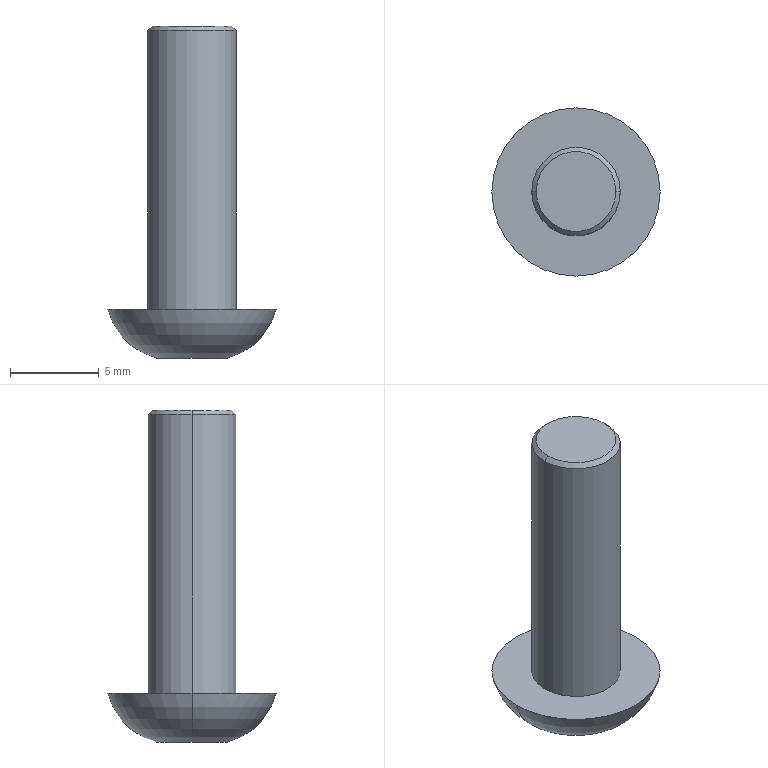Part | NX | features BREP 1 | 1 solid | 23 faces | box 9.5 x 9.5 x 18.75 mm | volume 434.554 mm3 | plane 15 | cone 4 | torus 2 | cylinder 2 | commonest cylinder face diameters 5 x2
STEP:
#1=CARTESIAN_POINT('',(0.,0.,-0.324));
#2=VERTEX_POINT('',#1);
#3=CARTESIAN_POINT('',(-1.5,0.,-1.19));
#4=VERTEX_POINT('',#3);
#5=CARTESIAN_POINT('',(-1.5,0.,-1.19));
#6=DIRECTION('',(-0.866,0.,-0.5));
#7=VECTOR('',#6,1000.);
#8=LINE('',#5,#7);
#9=EDGE_CURVE('',#2,#4,#8,.T.);
#10=ORIENTED_EDGE('',*,*,#9,.F.);
#11=CARTESIAN_POINT('',(1.5,0.,-1.19));
#12=VERTEX_POINT('',#11);
#13=CARTESIAN_POINT('',(1.5,0.,-1.19));
#14=DIRECTION('',(0.866,0.,-0.5));
#15=VECTOR('',#14,1000.);
#16=LINE('',#13,#15);
#17=EDGE_CURVE('',#2,#12,#16,.T.);
#18=ORIENTED_EDGE('',*,*,#17,.T.);
#19=CARTESIAN_POINT('',(1.299,-0.75,-1.19));
#20=VERTEX_POINT('',#19);
#21=CARTESIAN_POINT('',(0.,0.,-1.19));
#22=DIRECTION('',(0.,0.,1.));
#23=DIRECTION('',(1.,0.,0.));
#24=AXIS2_PLACEMENT_3D('',#21,#22,#23);
#25=CIRCLE('',#24,1.5);
#26=EDGE_CURVE('',#20,#12,#25,.T.);
#27=ORIENTED_EDGE('',*,*,#26,.F.);
#28=CARTESIAN_POINT('',(0.,-1.5,-1.19));
#29=VERTEX_POINT('',#28);
#30=CARTESIAN_POINT('',(0.,0.,-1.19));
#31=DIRECTION('',(0.,0.,1.));
#32=DIRECTION('',(1.,0.,0.));
#33=AXIS2_PLACEMENT_3D('',#30,#31,#32);
#34=CIRCLE('',#33,1.5);
#35=EDGE_CURVE('',#29,#20,#34,.T.);
#36=ORIENTED_EDGE('',*,*,#35,.F.);
#37=CARTESIAN_POINT('',(-1.299,-0.75,-1.19));
#38=VERTEX_POINT('',#37);
#39=CARTESIAN_POINT('',(0.,0.,-1.19));
#40=DIRECTION('',(0.,0.,1.));
#41=DIRECTION('',(1.,0.,0.));
#42=AXIS2_PLACEMENT_3D('',#39,#40,#41);
#43=CIRCLE('',#42,1.5);
#44=EDGE_CURVE('',#38,#29,#43,.T.);
#45=ORIENTED_EDGE('',*,*,#44,.F.);
#46=CARTESIAN_POINT('',(0.,0.,-1.19));
#47=DIRECTION('',(0.,0.,1.));
#48=DIRECTION('',(1.,0.,0.));
#49=AXIS2_PLACEMENT_3D('',#46,#47,#48);
#50=CIRCLE('',#49,1.5);
#51=EDGE_CURVE('',#4,#38,#50,.T.);
#52=ORIENTED_EDGE('',*,*,#51,.F.);
#53=EDGE_LOOP('',(#10,#18,#27,#36,#45,#52));
#54=FACE_BOUND('',#53,.T.);
#55=CARTESIAN_POINT('',(0.,0.,-1.19));
#56=DIRECTION('',(0.,0.,-1.));
#57=DIRECTION('',(-1.,0.,0.));
#58=AXIS2_PLACEMENT_3D('',#55,#56,#57);
#59=CONICAL_SURFACE('',#58,1.5,1.047);
#60=ADVANCED_FACE('',(#54),#59,.F.);
#61=CARTESIAN_POINT('',(2.25,0.,16.));
#62=VERTEX_POINT('',#61);
#63=CARTESIAN_POINT('',(-2.25,0.,16.));
#64=VERTEX_POINT('',#63);
#65=CARTESIAN_POINT('',(0.,0.,16.));
#66=DIRECTION('',(0.,0.,1.));
#67=DIRECTION('',(-1.,0.,0.));
#68=AXIS2_PLACEMENT_3D('',#65,#66,#67);
#69=CIRCLE('',#68,2.25);
#70=EDGE_CURVE('',#62,#64,#69,.T.);
#71=ORIENTED_EDGE('',*,*,#70,.F.);
#72=CARTESIAN_POINT('',(2.5,0.,15.75));
#73=VERTEX_POINT('',#72);
#74=CARTESIAN_POINT('',(2.5,0.,15.75));
#75=DIRECTION('',(0.7071,0.,-0.7071));
#76=VECTOR('',#75,1000.);
#77=LINE('',#74,#76);
#78=EDGE_CURVE('',#62,#73,#77,.T.);
#79=ORIENTED_EDGE('',*,*,#78,.T.);
#80=CARTESIAN_POINT('',(-2.5,0.,15.75));
#81=VERTEX_POINT('',#80);
#82=CARTESIAN_POINT('',(0.,0.,15.75));
#83=DIRECTION('',(0.,0.,-1.));
#84=DIRECTION('',(-1.,0.,0.));
#85=AXIS2_PLACEMENT_3D('',#82,#83,#84);
#86=CIRCLE('',#85,2.5);
#87=EDGE_CURVE('',#81,#73,#86,.T.);
#88=ORIENTED_EDGE('',*,*,#87,.F.);
#89=CARTESIAN_POINT('',(-2.5,0.,15.75));
#90=DIRECTION('',(-0.7071,0.,-0.7071));
#91=VECTOR('',#90,1000.);
#92=LINE('',#89,#91);
#93=EDGE_CURVE('',#64,#81,#92,.T.);
#94=ORIENTED_EDGE('',*,*,#93,.F.);
#95=EDGE_LOOP('',(#71,#79,#88,#94));
#96=FACE_BOUND('',#95,.T.);
#97=CARTESIAN_POINT('',(0.,0.,15.75));
#98=DIRECTION('',(0.,0.,-1.));
#99=DIRECTION('',(-1.,0.,0.));
#100=AXIS2_PLACEMENT_3D('',#97,#98,#99);
#101=CONICAL_SURFACE('',#100,2.5,0.7854);
#102=ADVANCED_FACE('',(#96),#101,.T.);
#103=CARTESIAN_POINT('',(-4.75,0.,0.));
#104=VERTEX_POINT('',#103);
#105=CARTESIAN_POINT('',(4.75,0.,0.));
#106=VERTEX_POINT('',#105);
#107=CARTESIAN_POINT('',(0.,0.,0.));
#108=DIRECTION('',(0.,0.,-1.));
#109=DIRECTION('',(-1.,0.,0.));
#110=AXIS2_PLACEMENT_3D('',#107,#108,#109);
#111=CIRCLE('',#110,4.75);
#112=EDGE_CURVE('',#104,#106,#111,.T.);
#113=ORIENTED_EDGE('',*,*,#112,.T.);
#114=CARTESIAN_POINT('',(2.,0.,-2.75));
#115=VERTEX_POINT('',#114);
#116=CARTESIAN_POINT('',(1.066,0.,0.9335));
#117=DIRECTION('',(0.,1.,0.));
#118=DIRECTION('',(-1.,0.,0.));
#119=AXIS2_PLACEMENT_3D('',#116,#117,#118);
#120=CIRCLE('',#119,3.8);
#121=EDGE_CURVE('',#106,#115,#120,.T.);
#122=ORIENTED_EDGE('',*,*,#121,.T.);
#123=CARTESIAN_POINT('',(-2.,0.,-2.75));
#124=VERTEX_POINT('',#123);
#125=CARTESIAN_POINT('',(0.,0.,-2.75));
#126=DIRECTION('',(0.,0.,-1.));
#127=DIRECTION('',(-1.,0.,0.));
#128=AXIS2_PLACEMENT_3D('',#125,#126,#127);
#129=CIRCLE('',#128,2.);
#130=EDGE_CURVE('',#124,#115,#129,.T.);
#131=ORIENTED_EDGE('',*,*,#130,.F.);
#132=CARTESIAN_POINT('',(-1.066,0.,0.9335));
#133=DIRECTION('',(0.,-1.,0.));
#134=DIRECTION('',(0.,0.,-1.));
#135=AXIS2_PLACEMENT_3D('',#132,#133,#134);
#136=CIRCLE('',#135,3.8);
#137=EDGE_CURVE('',#104,#124,#136,.T.);
#138=ORIENTED_EDGE('',*,*,#137,.F.);
#139=EDGE_LOOP('',(#113,#122,#131,#138));
#140=FACE_BOUND('',#139,.T.);
#141=CARTESIAN_POINT('',(0.,0.,0.9335));
#142=DIRECTION('',(0.,0.,-1.));
#143=DIRECTION('',(-1.,0.,0.));
#144=AXIS2_PLACEMENT_3D('',#141,#142,#143);
#145=DEGENERATE_TOROIDAL_SURFACE('',#144,1.066,3.8,.T.);
#146=ADVANCED_FACE('',(#140),#145,.T.);
#147=ORIENTED_EDGE('',*,*,#87,.T.);
#148=CARTESIAN_POINT('',(2.5,0.,0.));
#149=VERTEX_POINT('',#148);
#150=CARTESIAN_POINT('',(2.5,0.,16.));
#151=DIRECTION('',(0.,0.,-1.));
#152=VECTOR('',#151,1000.);
#153=LINE('',#150,#152);
#154=EDGE_CURVE('',#73,#149,#153,.T.);
#155=ORIENTED_EDGE('',*,*,#154,.T.);
#156=CARTESIAN_POINT('',(-2.5,0.,0.));
#157=VERTEX_POINT('',#156);
#158=CARTESIAN_POINT('',(0.,0.,0.));
#159=DIRECTION('',(0.,0.,1.));
#160=DIRECTION('',(1.,0.,0.));
#161=AXIS2_PLACEMENT_3D('',#158,#159,#160);
#162=CIRCLE('',#161,2.5);
#163=EDGE_CURVE('',#149,#157,#162,.T.);
#164=ORIENTED_EDGE('',*,*,#163,.T.);
#165=CARTESIAN_POINT('',(-2.5,0.,16.));
#166=DIRECTION('',(0.,0.,-1.));
#167=VECTOR('',#166,1000.);
#168=LINE('',#165,#167);
#169=EDGE_CURVE('',#81,#157,#168,.T.);
#170=ORIENTED_EDGE('',*,*,#169,.F.);
#171=EDGE_LOOP('',(#147,#155,#164,#170));
#172=FACE_BOUND('',#171,.T.);
#173=CARTESIAN_POINT('',(0.,0.,16.));
#174=DIRECTION('',(0.,0.,-1.));
#175=DIRECTION('',(-1.,0.,0.));
#176=AXIS2_PLACEMENT_3D('',#173,#174,#175);
#177=CYLINDRICAL_SURFACE('',#176,2.5);
#178=ADVANCED_FACE('',(#172),#177,.T.);
#179=CARTESIAN_POINT('',(1.299,0.75,-1.19));
#180=VERTEX_POINT('',#179);
#181=CARTESIAN_POINT('',(0.866,1.5,-1.19));
#182=VERTEX_POINT('',#181);
#183=CARTESIAN_POINT('',(1.732,0.,-1.19));
#184=DIRECTION('',(-0.5,0.866,0.));
#185=VECTOR('',#184,1000.);
#186=LINE('',#183,#185);
#187=EDGE_CURVE('',#180,#182,#186,.T.);
#188=ORIENTED_EDGE('',*,*,#187,.F.);
#189=CARTESIAN_POINT('',(0.,1.5,-1.19));
#190=VERTEX_POINT('',#189);
#191=CARTESIAN_POINT('',(0.,0.,-1.19));
#192=DIRECTION('',(0.,0.,1.));
#193=DIRECTION('',(1.,0.,0.));
#194=AXIS2_PLACEMENT_3D('',#191,#192,#193);
#195=CIRCLE('',#194,1.5);
#196=EDGE_CURVE('',#180,#190,#195,.T.);
#197=ORIENTED_EDGE('',*,*,#196,.T.);
#198=CARTESIAN_POINT('',(0.866,1.5,-1.19));
#199=DIRECTION('',(-1.,0.,0.));
#200=VECTOR('',#199,1000.);
#201=LINE('',#198,#200);
#202=EDGE_CURVE('',#182,#190,#201,.T.);
#203=ORIENTED_EDGE('',*,*,#202,.F.);
#204=EDGE_LOOP('',(#188,#197,#203));
#205=FACE_BOUND('',#204,.T.);
#206=CARTESIAN_POINT('',(0.,0.,-1.19));
#207=DIRECTION('',(0.,0.,1.));
#208=DIRECTION('',(1.,0.,0.));
#209=AXIS2_PLACEMENT_3D('',#206,#207,#208);
#210=PLANE('',#209);
#211=ADVANCED_FACE('',(#205),#210,.F.);
#212=CARTESIAN_POINT('',(-0.866,1.5,-1.19));
#213=VERTEX_POINT('',#212);
#214=CARTESIAN_POINT('',(0.866,1.5,-1.19));
#215=DIRECTION('',(-1.,0.,0.));
#216=VECTOR('',#215,1000.);
#217=LINE('',#214,#216);
#218=EDGE_CURVE('',#190,#213,#217,.T.);
#219=ORIENTED_EDGE('',*,*,#218,.F.);
#220=CARTESIAN_POINT('',(-1.299,0.75,-1.19));
#221=VERTEX_POINT('',#220);
#222=CARTESIAN_POINT('',(0.,0.,-1.19));
#223=DIRECTION('',(0.,0.,-1.));
#224=DIRECTION('',(-1.,0.,0.));
#225=AXIS2_PLACEMENT_3D('',#222,#223,#224);
#226=CIRCLE('',#225,1.5);
#227=EDGE_CURVE('',#221,#190,#226,.T.);
#228=ORIENTED_EDGE('',*,*,#227,.F.);
#229=CARTESIAN_POINT('',(-0.866,1.5,-1.19));
#230=DIRECTION('',(-0.5,-0.866,0.));
#231=VECTOR('',#230,1000.);
#232=LINE('',#229,#231);
#233=EDGE_CURVE('',#213,#221,#232,.T.);
#234=ORIENTED_EDGE('',*,*,#233,.F.);
#235=EDGE_LOOP('',(#219,#228,#234));
#236=FACE_BOUND('',#235,.T.);
#237=CARTESIAN_POINT('',(0.,0.,-1.19));
#238=DIRECTION('',(0.,0.,1.));
#239=DIRECTION('',(1.,0.,0.));
#240=AXIS2_PLACEMENT_3D('',#237,#238,#239);
#241=PLANE('',#240);
#242=ADVANCED_FACE('',(#236),#241,.F.);
#243=CARTESIAN_POINT('',(-1.732,0.,-1.19));
#244=VERTEX_POINT('',#243);
#245=CARTESIAN_POINT('',(-0.866,1.5,-1.19));
#246=DIRECTION('',(-0.5,-0.866,0.));
#247=VECTOR('',#246,1000.);
#248=LINE('',#245,#247);
#249=EDGE_CURVE('',#221,#244,#248,.T.);
#250=ORIENTED_EDGE('',*,*,#249,.F.);
#251=CARTESIAN_POINT('',(0.,0.,-1.19));
#252=DIRECTION('',(0.,0.,1.));
#253=DIRECTION('',(1.,0.,0.));
#254=AXIS2_PLACEMENT_3D('',#251,#252,#253);
#255=CIRCLE('',#254,1.5);
#256=EDGE_CURVE('',#221,#4,#255,.T.);
#257=ORIENTED_EDGE('',*,*,#256,.T.);
#258=ORIENTED_EDGE('',*,*,#51,.T.);
#259=CARTESIAN_POINT('',(-1.732,0.,-1.19));
#260=DIRECTION('',(0.5,-0.866,0.));
#261=VECTOR('',#260,1000.);
#262=LINE('',#259,#261);
#263=EDGE_CURVE('',#244,#38,#262,.T.);
#264=ORIENTED_EDGE('',*,*,#263,.F.);
#265=EDGE_LOOP('',(#250,#257,#258,#264));
#266=FACE_BOUND('',#265,.T.);
#267=CARTESIAN_POINT('',(0.,0.,-1.19));
#268=DIRECTION('',(0.,0.,1.));
#269=DIRECTION('',(1.,0.,0.));
#270=AXIS2_PLACEMENT_3D('',#267,#268,#269);
#271=PLANE('',#270);
#272=ADVANCED_FACE('',(#266),#271,.F.);
#273=CARTESIAN_POINT('',(-0.866,-1.5,-1.19));
#274=VERTEX_POINT('',#273);
#275=CARTESIAN_POINT('',(-1.732,0.,-1.19));
#276=DIRECTION('',(0.5,-0.866,0.));
#277=VECTOR('',#276,1000.);
#278=LINE('',#275,#277);
#279=EDGE_CURVE('',#38,#274,#278,.T.);
#280=ORIENTED_EDGE('',*,*,#279,.F.);
#281=ORIENTED_EDGE('',*,*,#44,.T.);
#282=CARTESIAN_POINT('',(-0.866,-1.5,-1.19));
#283=DIRECTION('',(1.,0.,0.));
#284=VECTOR('',#283,1000.);
#285=LINE('',#282,#284);
#286=EDGE_CURVE('',#274,#29,#285,.T.);
#287=ORIENTED_EDGE('',*,*,#286,.F.);
#288=EDGE_LOOP('',(#280,#281,#287));
#289=FACE_BOUND('',#288,.T.);
#290=CARTESIAN_POINT('',(0.,0.,-1.19));
#291=DIRECTION('',(0.,0.,1.));
#292=DIRECTION('',(1.,0.,0.));
#293=AXIS2_PLACEMENT_3D('',#290,#291,#292);
#294=PLANE('',#293);
#295=ADVANCED_FACE('',(#289),#294,.F.);
#296=CARTESIAN_POINT('',(0.866,-1.5,-1.19));
#297=VERTEX_POINT('',#296);
#298=CARTESIAN_POINT('',(-0.866,-1.5,-1.19));
#299=DIRECTION('',(1.,0.,0.));
#300=VECTOR('',#299,1000.);
#301=LINE('',#298,#300);
#302=EDGE_CURVE('',#29,#297,#301,.T.);
#303=ORIENTED_EDGE('',*,*,#302,.F.);
#304=ORIENTED_EDGE('',*,*,#35,.T.);
#305=CARTESIAN_POINT('',(0.866,-1.5,-1.19));
#306=DIRECTION('',(0.5,0.866,0.));
#307=VECTOR('',#306,1000.);
#308=LINE('',#305,#307);
#309=EDGE_CURVE('',#297,#20,#308,.T.);
#310=ORIENTED_EDGE('',*,*,#309,.F.);
#311=EDGE_LOOP('',(#303,#304,#310));
#312=FACE_BOUND('',#311,.T.);
#313=CARTESIAN_POINT('',(0.,0.,-1.19));
#314=DIRECTION('',(0.,0.,1.));
#315=DIRECTION('',(1.,0.,0.));
#316=AXIS2_PLACEMENT_3D('',#313,#314,#315);
#317=PLANE('',#316);
#318=ADVANCED_FACE('',(#312),#317,.F.);
#319=ORIENTED_EDGE('',*,*,#130,.T.);
#320=CARTESIAN_POINT('',(0.,0.,-2.75));
#321=DIRECTION('',(0.,0.,-1.));
#322=DIRECTION('',(-1.,0.,0.));
#323=AXIS2_PLACEMENT_3D('',#320,#321,#322);
#324=CIRCLE('',#323,2.);
#325=EDGE_CURVE('',#115,#124,#324,.T.);
#326=ORIENTED_EDGE('',*,*,#325,.T.);
#327=EDGE_LOOP('',(#319,#326));
#328=FACE_BOUND('',#327,.T.);
#329=CARTESIAN_POINT('',(1.732,0.,-2.75));
#330=VERTEX_POINT('',#329);
#331=CARTESIAN_POINT('',(0.866,1.5,-2.75));
#332=VERTEX_POINT('',#331);
#333=CARTESIAN_POINT('',(1.732,0.,-2.75));
#334=DIRECTION('',(-0.5,0.866,0.));
#335=VECTOR('',#334,1000.);
#336=LINE('',#333,#335);
#337=EDGE_CURVE('',#330,#332,#336,.T.);
#338=ORIENTED_EDGE('',*,*,#337,.T.);
#339=CARTESIAN_POINT('',(-0.866,1.5,-2.75));
#340=VERTEX_POINT('',#339);
#341=CARTESIAN_POINT('',(0.866,1.5,-2.75));
#342=DIRECTION('',(-1.,0.,0.));
#343=VECTOR('',#342,1000.);
#344=LINE('',#341,#343);
#345=EDGE_CURVE('',#332,#340,#344,.T.);
#346=ORIENTED_EDGE('',*,*,#345,.T.);
#347=CARTESIAN_POINT('',(-1.732,0.,-2.75));
#348=VERTEX_POINT('',#347);
#349=CARTESIAN_POINT('',(-0.866,1.5,-2.75));
#350=DIRECTION('',(-0.5,-0.866,0.));
#351=VECTOR('',#350,1000.);
#352=LINE('',#349,#351);
#353=EDGE_CURVE('',#340,#348,#352,.T.);
#354=ORIENTED_EDGE('',*,*,#353,.T.);
#355=CARTESIAN_POINT('',(-0.866,-1.5,-2.75));
#356=VERTEX_POINT('',#355);
#357=CARTESIAN_POINT('',(-1.732,0.,-2.75));
#358=DIRECTION('',(0.5,-0.866,0.));
#359=VECTOR('',#358,1000.);
#360=LINE('',#357,#359);
#361=EDGE_CURVE('',#348,#356,#360,.T.);
#362=ORIENTED_EDGE('',*,*,#361,.T.);
#363=CARTESIAN_POINT('',(0.866,-1.5,-2.75));
#364=VERTEX_POINT('',#363);
#365=CARTESIAN_POINT('',(-0.866,-1.5,-2.75));
#366=DIRECTION('',(1.,0.,0.));
#367=VECTOR('',#366,1000.);
#368=LINE('',#365,#367);
#369=EDGE_CURVE('',#356,#364,#368,.T.);
#370=ORIENTED_EDGE('',*,*,#369,.T.);
#371=CARTESIAN_POINT('',(0.866,-1.5,-2.75));
#372=DIRECTION('',(0.5,0.866,0.));
#373=VECTOR('',#372,1000.);
#374=LINE('',#371,#373);
#375=EDGE_CURVE('',#364,#330,#374,.T.);
#376=ORIENTED_EDGE('',*,*,#375,.T.);
#377=EDGE_LOOP('',(#338,#346,#354,#362,#370,#376));
#378=FACE_BOUND('',#377,.T.);
#379=CARTESIAN_POINT('',(0.,0.,-2.75));
#380=DIRECTION('',(0.,0.,1.));
#381=DIRECTION('',(1.,0.,0.));
#382=AXIS2_PLACEMENT_3D('',#379,#380,#381);
#383=PLANE('',#382);
#384=ADVANCED_FACE('',(#328,#378),#383,.F.);
#385=ORIENTED_EDGE('',*,*,#112,.F.);
#386=CARTESIAN_POINT('',(0.,0.,0.));
#387=DIRECTION('',(0.,0.,-1.));
#388=DIRECTION('',(-1.,0.,0.));
#389=AXIS2_PLACEMENT_3D('',#386,#387,#388);
#390=CIRCLE('',#389,4.75);
#391=EDGE_CURVE('',#106,#104,#390,.T.);
#392=ORIENTED_EDGE('',*,*,#391,.F.);
#393=EDGE_LOOP('',(#385,#392));
#394=FACE_BOUND('',#393,.T.);
#395=CARTESIAN_POINT('',(0.,0.,0.));
#396=DIRECTION('',(0.,0.,1.));
#397=DIRECTION('',(1.,0.,0.));
#398=AXIS2_PLACEMENT_3D('',#395,#396,#397);
#399=CIRCLE('',#398,2.5);
#400=EDGE_CURVE('',#157,#149,#399,.T.);
#401=ORIENTED_EDGE('',*,*,#400,.F.);
#402=ORIENTED_EDGE('',*,*,#163,.F.);
#403=EDGE_LOOP('',(#401,#402));
#404=FACE_BOUND('',#403,.T.);
#405=CARTESIAN_POINT('',(0.,0.,0.));
#406=DIRECTION('',(0.,0.,1.));
#407=DIRECTION('',(1.,0.,0.));
#408=AXIS2_PLACEMENT_3D('',#405,#406,#407);
#409=PLANE('',#408);
#410=ADVANCED_FACE('',(#394,#404),#409,.T.);
#411=ORIENTED_EDGE('',*,*,#154,.F.);
#412=CARTESIAN_POINT('',(0.,0.,15.75));
#413=DIRECTION('',(0.,0.,-1.));
#414=DIRECTION('',(-1.,0.,0.));
#415=AXIS2_PLACEMENT_3D('',#412,#413,#414);
#416=CIRCLE('',#415,2.5);
#417=EDGE_CURVE('',#73,#81,#416,.T.);
#418=ORIENTED_EDGE('',*,*,#417,.T.);
#419=ORIENTED_EDGE('',*,*,#169,.T.);
#420=ORIENTED_EDGE('',*,*,#400,.T.);
#421=EDGE_LOOP('',(#411,#418,#419,#420));
#422=FACE_BOUND('',#421,.T.);
#423=CARTESIAN_POINT('',(0.,0.,16.));
#424=DIRECTION('',(0.,0.,-1.));
#425=DIRECTION('',(-1.,0.,0.));
#426=AXIS2_PLACEMENT_3D('',#423,#424,#425);
#427=CYLINDRICAL_SURFACE('',#426,2.5);
#428=ADVANCED_FACE('',(#422),#427,.T.);
#429=CARTESIAN_POINT('',(0.,0.,16.));
#430=DIRECTION('',(0.,0.,1.));
#431=DIRECTION('',(-1.,0.,0.));
#432=AXIS2_PLACEMENT_3D('',#429,#430,#431);
#433=CIRCLE('',#432,2.25);
#434=EDGE_CURVE('',#64,#62,#433,.T.);
#435=ORIENTED_EDGE('',*,*,#434,.T.);
#436=ORIENTED_EDGE('',*,*,#70,.T.);
#437=EDGE_LOOP('',(#435,#436));
#438=FACE_BOUND('',#437,.T.);
#439=CARTESIAN_POINT('',(0.,0.,16.));
#440=DIRECTION('',(0.,0.,-1.));
#441=DIRECTION('',(0.,-1.,0.));
#442=AXIS2_PLACEMENT_3D('',#439,#440,#441);
#443=PLANE('',#442);
#444=ADVANCED_FACE('',(#438),#443,.F.);
#445=ORIENTED_EDGE('',*,*,#121,.F.);
#446=ORIENTED_EDGE('',*,*,#391,.T.);
#447=ORIENTED_EDGE('',*,*,#137,.T.);
#448=ORIENTED_EDGE('',*,*,#325,.F.);
#449=EDGE_LOOP('',(#445,#446,#447,#448));
#450=FACE_BOUND('',#449,.T.);
#451=CARTESIAN_POINT('',(0.,0.,0.9335));
#452=DIRECTION('',(0.,0.,-1.));
#453=DIRECTION('',(-1.,0.,0.));
#454=AXIS2_PLACEMENT_3D('',#451,#452,#453);
#455=DEGENERATE_TOROIDAL_SURFACE('',#454,1.066,3.8,.T.);
#456=ADVANCED_FACE('',(#450),#455,.T.);
#457=ORIENTED_EDGE('',*,*,#78,.F.);
#458=ORIENTED_EDGE('',*,*,#434,.F.);
#459=ORIENTED_EDGE('',*,*,#93,.T.);
#460=ORIENTED_EDGE('',*,*,#417,.F.);
#461=EDGE_LOOP('',(#457,#458,#459,#460));
#462=FACE_BOUND('',#461,.T.);
#463=CARTESIAN_POINT('',(0.,0.,15.75));
#464=DIRECTION('',(0.,0.,-1.));
#465=DIRECTION('',(-1.,0.,0.));
#466=AXIS2_PLACEMENT_3D('',#463,#464,#465);
#467=CONICAL_SURFACE('',#466,2.5,0.7854);
#468=ADVANCED_FACE('',(#462),#467,.T.);
#469=ORIENTED_EDGE('',*,*,#337,.F.);
#470=CARTESIAN_POINT('',(1.732,0.,-1.19));
#471=VERTEX_POINT('',#470);
#472=CARTESIAN_POINT('',(1.732,0.,-1.19));
#473=DIRECTION('',(0.,0.,-1.));
#474=VECTOR('',#473,1000.);
#475=LINE('',#472,#474);
#476=EDGE_CURVE('',#471,#330,#475,.T.);
#477=ORIENTED_EDGE('',*,*,#476,.F.);
#478=CARTESIAN_POINT('',(1.732,0.,-1.19));
#479=DIRECTION('',(-0.5,0.866,0.));
#480=VECTOR('',#479,1000.);
#481=LINE('',#478,#480);
#482=EDGE_CURVE('',#471,#180,#481,.T.);
#483=ORIENTED_EDGE('',*,*,#482,.T.);
#484=ORIENTED_EDGE('',*,*,#187,.T.);
#485=CARTESIAN_POINT('',(0.866,1.5,-1.19));
#486=DIRECTION('',(0.,0.,-1.));
#487=VECTOR('',#486,1000.);
#488=LINE('',#485,#487);
#489=EDGE_CURVE('',#182,#332,#488,.T.);
#490=ORIENTED_EDGE('',*,*,#489,.T.);
#491=EDGE_LOOP('',(#469,#477,#483,#484,#490));
#492=FACE_BOUND('',#491,.T.);
#493=CARTESIAN_POINT('',(1.732,0.,-1.19));
#494=DIRECTION('',(-0.866,-0.5,0.));
#495=DIRECTION('',(-0.5,0.866,0.));
#496=AXIS2_PLACEMENT_3D('',#493,#494,#495);
#497=PLANE('',#496);
#498=ADVANCED_FACE('',(#492),#497,.T.);
#499=ORIENTED_EDGE('',*,*,#345,.F.);
#500=ORIENTED_EDGE('',*,*,#489,.F.);
#501=ORIENTED_EDGE('',*,*,#202,.T.);
#502=ORIENTED_EDGE('',*,*,#218,.T.);
#503=CARTESIAN_POINT('',(-0.866,1.5,-1.19));
#504=DIRECTION('',(0.,0.,-1.));
#505=VECTOR('',#504,1000.);
#506=LINE('',#503,#505);
#507=EDGE_CURVE('',#213,#340,#506,.T.);
#508=ORIENTED_EDGE('',*,*,#507,.T.);
#509=EDGE_LOOP('',(#499,#500,#501,#502,#508));
#510=FACE_BOUND('',#509,.T.);
#511=CARTESIAN_POINT('',(0.866,1.5,-1.19));
#512=DIRECTION('',(0.,-1.,0.));
#513=DIRECTION('',(0.,0.,-1.));
#514=AXIS2_PLACEMENT_3D('',#511,#512,#513);
#515=PLANE('',#514);
#516=ADVANCED_FACE('',(#510),#515,.T.);
#517=ORIENTED_EDGE('',*,*,#353,.F.);
#518=ORIENTED_EDGE('',*,*,#507,.F.);
#519=ORIENTED_EDGE('',*,*,#233,.T.);
#520=ORIENTED_EDGE('',*,*,#249,.T.);
#521=CARTESIAN_POINT('',(-1.732,0.,-1.19));
#522=DIRECTION('',(0.,0.,-1.));
#523=VECTOR('',#522,1000.);
#524=LINE('',#521,#523);
#525=EDGE_CURVE('',#244,#348,#524,.T.);
#526=ORIENTED_EDGE('',*,*,#525,.T.);
#527=EDGE_LOOP('',(#517,#518,#519,#520,#526));
#528=FACE_BOUND('',#527,.T.);
#529=CARTESIAN_POINT('',(-0.866,1.5,-1.19));
#530=DIRECTION('',(0.866,-0.5,0.));
#531=DIRECTION('',(0.,0.,-1.));
#532=AXIS2_PLACEMENT_3D('',#529,#530,#531);
#533=PLANE('',#532);
#534=ADVANCED_FACE('',(#528),#533,.T.);
#535=ORIENTED_EDGE('',*,*,#361,.F.);
#536=ORIENTED_EDGE('',*,*,#525,.F.);
#537=ORIENTED_EDGE('',*,*,#263,.T.);
#538=ORIENTED_EDGE('',*,*,#279,.T.);
#539=CARTESIAN_POINT('',(-0.866,-1.5,-1.19));
#540=DIRECTION('',(0.,0.,-1.));
#541=VECTOR('',#540,1000.);
#542=LINE('',#539,#541);
#543=EDGE_CURVE('',#274,#356,#542,.T.);
#544=ORIENTED_EDGE('',*,*,#543,.T.);
#545=EDGE_LOOP('',(#535,#536,#537,#538,#544));
#546=FACE_BOUND('',#545,.T.);
#547=CARTESIAN_POINT('',(-1.732,0.,-1.19));
#548=DIRECTION('',(0.866,0.5,0.));
#549=DIRECTION('',(0.,0.,-1.));
#550=AXIS2_PLACEMENT_3D('',#547,#548,#549);
#551=PLANE('',#550);
#552=ADVANCED_FACE('',(#546),#551,.T.);
#553=ORIENTED_EDGE('',*,*,#369,.F.);
#554=ORIENTED_EDGE('',*,*,#543,.F.);
#555=ORIENTED_EDGE('',*,*,#286,.T.);
#556=ORIENTED_EDGE('',*,*,#302,.T.);
#557=CARTESIAN_POINT('',(0.866,-1.5,-1.19));
#558=DIRECTION('',(0.,0.,-1.));
#559=VECTOR('',#558,1000.);
#560=LINE('',#557,#559);
#561=EDGE_CURVE('',#297,#364,#560,.T.);
#562=ORIENTED_EDGE('',*,*,#561,.T.);
#563=EDGE_LOOP('',(#553,#554,#555,#556,#562));
#564=FACE_BOUND('',#563,.T.);
#565=CARTESIAN_POINT('',(-0.866,-1.5,-1.19));
#566=DIRECTION('',(0.,1.,0.));
#567=DIRECTION('',(1.,0.,0.));
#568=AXIS2_PLACEMENT_3D('',#565,#566,#567);
#569=PLANE('',#568);
#570=ADVANCED_FACE('',(#564),#569,.T.);
#571=ORIENTED_EDGE('',*,*,#375,.F.);
#572=ORIENTED_EDGE('',*,*,#561,.F.);
#573=ORIENTED_EDGE('',*,*,#309,.T.);
#574=CARTESIAN_POINT('',(0.866,-1.5,-1.19));
#575=DIRECTION('',(0.5,0.866,0.));
#576=VECTOR('',#575,1000.);
#577=LINE('',#574,#576);
#578=EDGE_CURVE('',#20,#471,#577,.T.);
#579=ORIENTED_EDGE('',*,*,#578,.T.);
#580=ORIENTED_EDGE('',*,*,#476,.T.);
#581=EDGE_LOOP('',(#571,#572,#573,#579,#580));
#582=FACE_BOUND('',#581,.T.);
#583=CARTESIAN_POINT('',(0.866,-1.5,-1.19));
#584=DIRECTION('',(-0.866,0.5,0.));
#585=DIRECTION('',(0.,0.,1.));
#586=AXIS2_PLACEMENT_3D('',#583,#584,#585);
#587=PLANE('',#586);
#588=ADVANCED_FACE('',(#582),#587,.T.);
#589=ORIENTED_EDGE('',*,*,#578,.F.);
#590=ORIENTED_EDGE('',*,*,#26,.T.);
#591=CARTESIAN_POINT('',(0.,0.,-1.19));
#592=DIRECTION('',(0.,0.,1.));
#593=DIRECTION('',(1.,0.,0.));
#594=AXIS2_PLACEMENT_3D('',#591,#592,#593);
#595=CIRCLE('',#594,1.5);
#596=EDGE_CURVE('',#12,#180,#595,.T.);
#597=ORIENTED_EDGE('',*,*,#596,.T.);
#598=ORIENTED_EDGE('',*,*,#482,.F.);
#599=EDGE_LOOP('',(#589,#590,#597,#598));
#600=FACE_BOUND('',#599,.T.);
#601=CARTESIAN_POINT('',(0.,0.,-1.19));
#602=DIRECTION('',(0.,0.,1.));
#603=DIRECTION('',(1.,0.,0.));
#604=AXIS2_PLACEMENT_3D('',#601,#602,#603);
#605=PLANE('',#604);
#606=ADVANCED_FACE('',(#600),#605,.F.);
#607=ORIENTED_EDGE('',*,*,#17,.F.);
#608=ORIENTED_EDGE('',*,*,#9,.T.);
#609=ORIENTED_EDGE('',*,*,#256,.F.);
#610=ORIENTED_EDGE('',*,*,#227,.T.);
#611=ORIENTED_EDGE('',*,*,#196,.F.);
#612=ORIENTED_EDGE('',*,*,#596,.F.);
#613=EDGE_LOOP('',(#607,#608,#609,#610,#611,#612));
#614=FACE_BOUND('',#613,.T.);
#615=CARTESIAN_POINT('',(0.,0.,-1.19));
#616=DIRECTION('',(0.,0.,-1.));
#617=DIRECTION('',(-1.,0.,0.));
#618=AXIS2_PLACEMENT_3D('',#615,#616,#617);
#619=CONICAL_SURFACE('',#618,1.5,1.047);
#620=ADVANCED_FACE('',(#614),#619,.F.);
#621=CLOSED_SHELL('',(#60,#102,#146,#178,#211,#242,#272,#295,#318,#384,#410,#428,#444,#456,#468,#498,#516,#534,#552,#570,#588,#606,#620));
#622=MANIFOLD_SOLID_BREP('',#621);
#623=(LENGTH_UNIT()NAMED_UNIT(*)SI_UNIT(.MILLI.,.METRE.));
#624=UNCERTAINTY_MEASURE_WITH_UNIT(LENGTH_MEASURE(0.00001),#623,'','');
#625=(NAMED_UNIT(*)PLANE_ANGLE_UNIT()SI_UNIT($,.RADIAN.));
#626=(NAMED_UNIT(*)SI_UNIT($,.STERADIAN.)SOLID_ANGLE_UNIT());
#627=(GEOMETRIC_REPRESENTATION_CONTEXT(3)GLOBAL_UNCERTAINTY_ASSIGNED_CONTEXT((#624))GLOBAL_UNIT_ASSIGNED_CONTEXT((#623,#625,#626))REPRESENTATION_CONTEXT('',''));
#628=ADVANCED_BREP_SHAPE_REPRESENTATION('',(#622),#627);